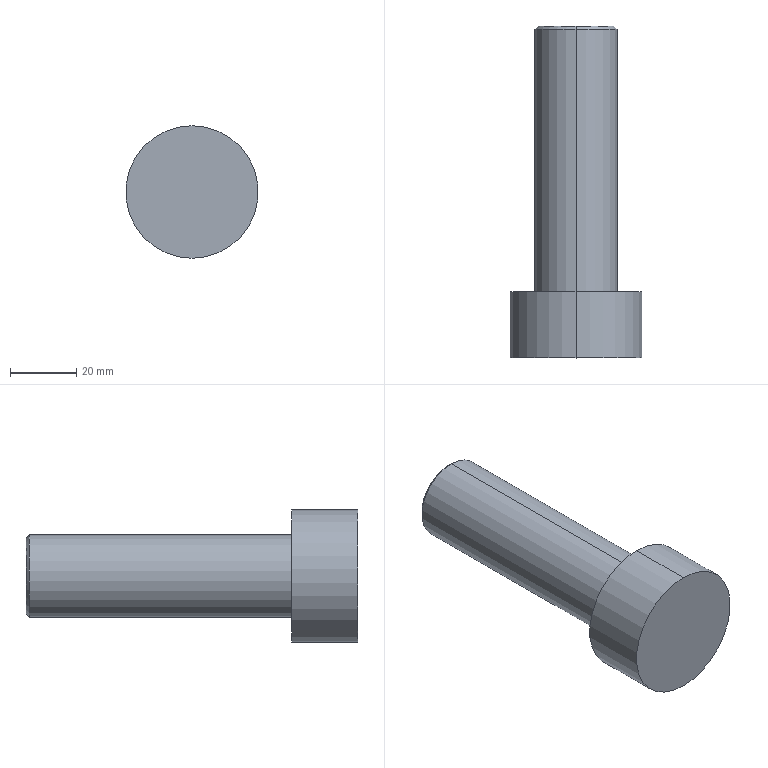Part | SolidWorks | features BaseBody 1, HoleWzd 1 | 1 solid | 13 faces | box 40 x 100.2 x 40 mm | volume 63721 mm3 | cylinder 6 | cone 4 | plane 3 | commonest cylinder face diameters 6.8 x2 25 x2 40 x2
STEP:
#1=CARTESIAN_POINT('',(0.,80.45,-3.4));
#2=VERTEX_POINT('',#1);
#3=CARTESIAN_POINT('',(0.,80.45,3.4));
#4=VERTEX_POINT('',#3);
#5=CARTESIAN_POINT('',(0.,80.45,0.));
#6=DIRECTION('',(0.,1.,0.));
#7=DIRECTION('',(0.,0.,1.));
#8=AXIS2_PLACEMENT_3D('',#5,#6,#7);
#9=CIRCLE('',#8,3.4);
#10=EDGE_CURVE('',#2,#4,#9,.T.);
#11=ORIENTED_EDGE('',*,*,#10,.F.);
#12=CARTESIAN_POINT('',(0.,100.2,-3.4));
#13=VERTEX_POINT('',#12);
#14=CARTESIAN_POINT('',(0.,100.2,-3.4));
#15=DIRECTION('',(0.,1.,0.));
#16=VECTOR('',#15,1000.);
#17=LINE('',#14,#16);
#18=EDGE_CURVE('',#2,#13,#17,.T.);
#19=ORIENTED_EDGE('',*,*,#18,.T.);
#20=CARTESIAN_POINT('',(0.,100.2,3.4));
#21=VERTEX_POINT('',#20);
#22=CARTESIAN_POINT('',(0.,100.2,0.));
#23=DIRECTION('',(0.,1.,0.));
#24=DIRECTION('',(0.,0.,1.));
#25=AXIS2_PLACEMENT_3D('',#22,#23,#24);
#26=CIRCLE('',#25,3.4);
#27=EDGE_CURVE('',#13,#21,#26,.T.);
#28=ORIENTED_EDGE('',*,*,#27,.T.);
#29=CARTESIAN_POINT('',(0.,100.2,3.4));
#30=DIRECTION('',(0.,1.,0.));
#31=VECTOR('',#30,1000.);
#32=LINE('',#29,#31);
#33=EDGE_CURVE('',#4,#21,#32,.T.);
#34=ORIENTED_EDGE('',*,*,#33,.F.);
#35=EDGE_LOOP('',(#11,#19,#28,#34));
#36=FACE_OUTER_BOUND('',#35,.T.);
#37=CARTESIAN_POINT('',(0.,100.2,0.));
#38=DIRECTION('',(0.,1.,0.));
#39=DIRECTION('',(0.,0.,1.));
#40=AXIS2_PLACEMENT_3D('',#37,#38,#39);
#41=CYLINDRICAL_SURFACE('',#40,3.4);
#42=ADVANCED_FACE('',(#36),#41,.F.);
#43=CARTESIAN_POINT('',(0.,78.407,0.));
#44=VERTEX_POINT('',#43);
#45=CARTESIAN_POINT('',(0.,80.45,3.4));
#46=DIRECTION('',(0.,0.515,0.8572));
#47=VECTOR('',#46,1000.);
#48=LINE('',#45,#47);
#49=EDGE_CURVE('',#44,#4,#48,.T.);
#50=ORIENTED_EDGE('',*,*,#49,.F.);
#51=CARTESIAN_POINT('',(0.,80.45,-3.4));
#52=DIRECTION('',(0.,0.515,-0.8572));
#53=VECTOR('',#52,1000.);
#54=LINE('',#51,#53);
#55=EDGE_CURVE('',#44,#2,#54,.T.);
#56=ORIENTED_EDGE('',*,*,#55,.T.);
#57=ORIENTED_EDGE('',*,*,#10,.T.);
#58=EDGE_LOOP('',(#50,#56,#57));
#59=FACE_OUTER_BOUND('',#58,.T.);
#60=CARTESIAN_POINT('',(0.,80.45,0.));
#61=DIRECTION('',(0.,1.,0.));
#62=DIRECTION('',(0.,0.,1.));
#63=AXIS2_PLACEMENT_3D('',#60,#61,#62);
#64=CONICAL_SURFACE('',#63,3.4,1.03);
#65=ADVANCED_FACE('',(#59),#64,.F.);
#66=CARTESIAN_POINT('',(0.,20.,12.5));
#67=VERTEX_POINT('',#66);
#68=CARTESIAN_POINT('',(0.,20.,-12.5));
#69=VERTEX_POINT('',#68);
#70=CARTESIAN_POINT('',(0.,20.,0.));
#71=DIRECTION('',(0.,1.,0.));
#72=DIRECTION('',(0.,0.,1.));
#73=AXIS2_PLACEMENT_3D('',#70,#71,#72);
#74=CIRCLE('',#73,12.5);
#75=EDGE_CURVE('',#67,#69,#74,.T.);
#76=ORIENTED_EDGE('',*,*,#75,.T.);
#77=CARTESIAN_POINT('',(0.,99.2,-12.5));
#78=VERTEX_POINT('',#77);
#79=CARTESIAN_POINT('',(0.,0.,-12.5));
#80=DIRECTION('',(0.,1.,0.));
#81=VECTOR('',#80,1000.);
#82=LINE('',#79,#81);
#83=EDGE_CURVE('',#69,#78,#82,.T.);
#84=ORIENTED_EDGE('',*,*,#83,.T.);
#85=CARTESIAN_POINT('',(0.,99.2,12.5));
#86=VERTEX_POINT('',#85);
#87=CARTESIAN_POINT('',(0.,99.2,0.));
#88=DIRECTION('',(0.,-1.,0.));
#89=DIRECTION('',(0.,0.,1.));
#90=AXIS2_PLACEMENT_3D('',#87,#88,#89);
#91=CIRCLE('',#90,12.5);
#92=EDGE_CURVE('',#78,#86,#91,.T.);
#93=ORIENTED_EDGE('',*,*,#92,.T.);
#94=CARTESIAN_POINT('',(0.,0.,12.5));
#95=DIRECTION('',(0.,1.,0.));
#96=VECTOR('',#95,1000.);
#97=LINE('',#94,#96);
#98=EDGE_CURVE('',#67,#86,#97,.T.);
#99=ORIENTED_EDGE('',*,*,#98,.F.);
#100=EDGE_LOOP('',(#76,#84,#93,#99));
#101=FACE_OUTER_BOUND('',#100,.T.);
#102=CARTESIAN_POINT('',(0.,0.,0.));
#103=DIRECTION('',(0.,1.,0.));
#104=DIRECTION('',(0.,0.,1.));
#105=AXIS2_PLACEMENT_3D('',#102,#103,#104);
#106=CYLINDRICAL_SURFACE('',#105,12.5);
#107=ADVANCED_FACE('',(#101),#106,.T.);
#108=CARTESIAN_POINT('',(0.,100.2,-11.5));
#109=VERTEX_POINT('',#108);
#110=CARTESIAN_POINT('',(0.,100.2,11.5));
#111=VERTEX_POINT('',#110);
#112=CARTESIAN_POINT('',(0.,100.2,0.));
#113=DIRECTION('',(0.,-1.,0.));
#114=DIRECTION('',(0.,0.,-1.));
#115=AXIS2_PLACEMENT_3D('',#112,#113,#114);
#116=CIRCLE('',#115,11.5);
#117=EDGE_CURVE('',#109,#111,#116,.T.);
#118=ORIENTED_EDGE('',*,*,#117,.T.);
#119=CARTESIAN_POINT('',(0.,99.2,12.5));
#120=DIRECTION('',(0.,-0.7071,0.7071));
#121=VECTOR('',#120,1000.);
#122=LINE('',#119,#121);
#123=EDGE_CURVE('',#111,#86,#122,.T.);
#124=ORIENTED_EDGE('',*,*,#123,.T.);
#125=ORIENTED_EDGE('',*,*,#92,.F.);
#126=CARTESIAN_POINT('',(0.,99.2,-12.5));
#127=DIRECTION('',(0.,-0.7071,-0.7071));
#128=VECTOR('',#127,1000.);
#129=LINE('',#126,#128);
#130=EDGE_CURVE('',#109,#78,#129,.T.);
#131=ORIENTED_EDGE('',*,*,#130,.F.);
#132=EDGE_LOOP('',(#118,#124,#125,#131));
#133=FACE_OUTER_BOUND('',#132,.T.);
#134=CARTESIAN_POINT('',(0.,99.2,0.));
#135=DIRECTION('',(0.,-1.,0.));
#136=DIRECTION('',(0.,0.,-1.));
#137=AXIS2_PLACEMENT_3D('',#134,#135,#136);
#138=CONICAL_SURFACE('',#137,12.5,0.7854);
#139=ADVANCED_FACE('',(#133),#138,.T.);
#140=CARTESIAN_POINT('',(0.,0.,20.));
#141=VERTEX_POINT('',#140);
#142=CARTESIAN_POINT('',(0.,0.,-20.));
#143=VERTEX_POINT('',#142);
#144=CARTESIAN_POINT('',(0.,0.,0.));
#145=DIRECTION('',(0.,1.,0.));
#146=DIRECTION('',(0.,0.,1.));
#147=AXIS2_PLACEMENT_3D('',#144,#145,#146);
#148=CIRCLE('',#147,20.);
#149=EDGE_CURVE('',#141,#143,#148,.T.);
#150=ORIENTED_EDGE('',*,*,#149,.T.);
#151=CARTESIAN_POINT('',(0.,20.,-20.));
#152=VERTEX_POINT('',#151);
#153=CARTESIAN_POINT('',(0.,0.,-20.));
#154=DIRECTION('',(0.,1.,0.));
#155=VECTOR('',#154,1000.);
#156=LINE('',#153,#155);
#157=EDGE_CURVE('',#143,#152,#156,.T.);
#158=ORIENTED_EDGE('',*,*,#157,.T.);
#159=CARTESIAN_POINT('',(0.,20.,20.));
#160=VERTEX_POINT('',#159);
#161=CARTESIAN_POINT('',(0.,20.,0.));
#162=DIRECTION('',(0.,-1.,0.));
#163=DIRECTION('',(0.,0.,1.));
#164=AXIS2_PLACEMENT_3D('',#161,#162,#163);
#165=CIRCLE('',#164,20.);
#166=EDGE_CURVE('',#152,#160,#165,.T.);
#167=ORIENTED_EDGE('',*,*,#166,.T.);
#168=CARTESIAN_POINT('',(0.,0.,20.));
#169=DIRECTION('',(0.,1.,0.));
#170=VECTOR('',#169,1000.);
#171=LINE('',#168,#170);
#172=EDGE_CURVE('',#141,#160,#171,.T.);
#173=ORIENTED_EDGE('',*,*,#172,.F.);
#174=EDGE_LOOP('',(#150,#158,#167,#173));
#175=FACE_OUTER_BOUND('',#174,.T.);
#176=CARTESIAN_POINT('',(0.,0.,0.));
#177=DIRECTION('',(0.,1.,0.));
#178=DIRECTION('',(0.,0.,1.));
#179=AXIS2_PLACEMENT_3D('',#176,#177,#178);
#180=CYLINDRICAL_SURFACE('',#179,20.);
#181=ADVANCED_FACE('',(#175),#180,.T.);
#182=ORIENTED_EDGE('',*,*,#83,.F.);
#183=CARTESIAN_POINT('',(0.,20.,0.));
#184=DIRECTION('',(0.,1.,0.));
#185=DIRECTION('',(0.,0.,1.));
#186=AXIS2_PLACEMENT_3D('',#183,#184,#185);
#187=CIRCLE('',#186,12.5);
#188=EDGE_CURVE('',#69,#67,#187,.T.);
#189=ORIENTED_EDGE('',*,*,#188,.T.);
#190=ORIENTED_EDGE('',*,*,#98,.T.);
#191=CARTESIAN_POINT('',(0.,99.2,0.));
#192=DIRECTION('',(0.,-1.,0.));
#193=DIRECTION('',(0.,0.,1.));
#194=AXIS2_PLACEMENT_3D('',#191,#192,#193);
#195=CIRCLE('',#194,12.5);
#196=EDGE_CURVE('',#86,#78,#195,.T.);
#197=ORIENTED_EDGE('',*,*,#196,.T.);
#198=EDGE_LOOP('',(#182,#189,#190,#197));
#199=FACE_OUTER_BOUND('',#198,.T.);
#200=CARTESIAN_POINT('',(0.,0.,0.));
#201=DIRECTION('',(0.,1.,0.));
#202=DIRECTION('',(0.,0.,1.));
#203=AXIS2_PLACEMENT_3D('',#200,#201,#202);
#204=CYLINDRICAL_SURFACE('',#203,12.5);
#205=ADVANCED_FACE('',(#199),#204,.T.);
#206=ORIENTED_EDGE('',*,*,#123,.F.);
#207=CARTESIAN_POINT('',(0.,100.2,0.));
#208=DIRECTION('',(0.,-1.,0.));
#209=DIRECTION('',(0.,0.,-1.));
#210=AXIS2_PLACEMENT_3D('',#207,#208,#209);
#211=CIRCLE('',#210,11.5);
#212=EDGE_CURVE('',#111,#109,#211,.T.);
#213=ORIENTED_EDGE('',*,*,#212,.T.);
#214=ORIENTED_EDGE('',*,*,#130,.T.);
#215=ORIENTED_EDGE('',*,*,#196,.F.);
#216=EDGE_LOOP('',(#206,#213,#214,#215));
#217=FACE_OUTER_BOUND('',#216,.T.);
#218=CARTESIAN_POINT('',(0.,99.2,0.));
#219=DIRECTION('',(0.,-1.,0.));
#220=DIRECTION('',(0.,0.,-1.));
#221=AXIS2_PLACEMENT_3D('',#218,#219,#220);
#222=CONICAL_SURFACE('',#221,12.5,0.7854);
#223=ADVANCED_FACE('',(#217),#222,.T.);
#224=ORIENTED_EDGE('',*,*,#75,.F.);
#225=ORIENTED_EDGE('',*,*,#188,.F.);
#226=EDGE_LOOP('',(#224,#225));
#227=FACE_BOUND('',#226,.T.);
#228=CARTESIAN_POINT('',(0.,20.,0.));
#229=DIRECTION('',(0.,-1.,0.));
#230=DIRECTION('',(0.,0.,1.));
#231=AXIS2_PLACEMENT_3D('',#228,#229,#230);
#232=CIRCLE('',#231,20.);
#233=EDGE_CURVE('',#160,#152,#232,.T.);
#234=ORIENTED_EDGE('',*,*,#233,.F.);
#235=ORIENTED_EDGE('',*,*,#166,.F.);
#236=EDGE_LOOP('',(#234,#235));
#237=FACE_OUTER_BOUND('',#236,.T.);
#238=CARTESIAN_POINT('',(12.5,20.,0.));
#239=DIRECTION('',(0.,-1.,0.));
#240=DIRECTION('',(0.,0.,-1.));
#241=AXIS2_PLACEMENT_3D('',#238,#239,#240);
#242=PLANE('',#241);
#243=ADVANCED_FACE('',(#227,#237),#242,.F.);
#244=CARTESIAN_POINT('',(0.,100.2,0.));
#245=DIRECTION('',(0.,1.,0.));
#246=DIRECTION('',(0.,0.,1.));
#247=AXIS2_PLACEMENT_3D('',#244,#245,#246);
#248=CIRCLE('',#247,3.4);
#249=EDGE_CURVE('',#21,#13,#248,.T.);
#250=ORIENTED_EDGE('',*,*,#249,.F.);
#251=ORIENTED_EDGE('',*,*,#27,.F.);
#252=EDGE_LOOP('',(#250,#251));
#253=FACE_BOUND('',#252,.T.);
#254=ORIENTED_EDGE('',*,*,#117,.F.);
#255=ORIENTED_EDGE('',*,*,#212,.F.);
#256=EDGE_LOOP('',(#254,#255));
#257=FACE_OUTER_BOUND('',#256,.T.);
#258=CARTESIAN_POINT('',(0.,100.2,0.));
#259=DIRECTION('',(0.,-1.,0.));
#260=DIRECTION('',(0.,0.,-1.));
#261=AXIS2_PLACEMENT_3D('',#258,#259,#260);
#262=PLANE('',#261);
#263=ADVANCED_FACE('',(#253,#257),#262,.F.);
#264=ORIENTED_EDGE('',*,*,#157,.F.);
#265=CARTESIAN_POINT('',(0.,0.,0.));
#266=DIRECTION('',(0.,1.,0.));
#267=DIRECTION('',(0.,0.,1.));
#268=AXIS2_PLACEMENT_3D('',#265,#266,#267);
#269=CIRCLE('',#268,20.);
#270=EDGE_CURVE('',#143,#141,#269,.T.);
#271=ORIENTED_EDGE('',*,*,#270,.T.);
#272=ORIENTED_EDGE('',*,*,#172,.T.);
#273=ORIENTED_EDGE('',*,*,#233,.T.);
#274=EDGE_LOOP('',(#264,#271,#272,#273));
#275=FACE_OUTER_BOUND('',#274,.T.);
#276=CARTESIAN_POINT('',(0.,0.,0.));
#277=DIRECTION('',(0.,1.,0.));
#278=DIRECTION('',(0.,0.,1.));
#279=AXIS2_PLACEMENT_3D('',#276,#277,#278);
#280=CYLINDRICAL_SURFACE('',#279,20.);
#281=ADVANCED_FACE('',(#275),#280,.T.);
#282=ORIENTED_EDGE('',*,*,#149,.F.);
#283=ORIENTED_EDGE('',*,*,#270,.F.);
#284=EDGE_LOOP('',(#282,#283));
#285=FACE_OUTER_BOUND('',#284,.T.);
#286=CARTESIAN_POINT('',(20.,0.,0.));
#287=DIRECTION('',(0.,1.,0.));
#288=DIRECTION('',(0.,0.,1.));
#289=AXIS2_PLACEMENT_3D('',#286,#287,#288);
#290=PLANE('',#289);
#291=ADVANCED_FACE('',(#285),#290,.F.);
#292=ORIENTED_EDGE('',*,*,#55,.F.);
#293=ORIENTED_EDGE('',*,*,#49,.T.);
#294=CARTESIAN_POINT('',(0.,80.45,0.));
#295=DIRECTION('',(0.,1.,0.));
#296=DIRECTION('',(0.,0.,1.));
#297=AXIS2_PLACEMENT_3D('',#294,#295,#296);
#298=CIRCLE('',#297,3.4);
#299=EDGE_CURVE('',#4,#2,#298,.T.);
#300=ORIENTED_EDGE('',*,*,#299,.T.);
#301=EDGE_LOOP('',(#292,#293,#300));
#302=FACE_OUTER_BOUND('',#301,.T.);
#303=CARTESIAN_POINT('',(0.,80.45,0.));
#304=DIRECTION('',(0.,1.,0.));
#305=DIRECTION('',(0.,0.,1.));
#306=AXIS2_PLACEMENT_3D('',#303,#304,#305);
#307=CONICAL_SURFACE('',#306,3.4,1.03);
#308=ADVANCED_FACE('',(#302),#307,.F.);
#309=ORIENTED_EDGE('',*,*,#18,.F.);
#310=ORIENTED_EDGE('',*,*,#299,.F.);
#311=ORIENTED_EDGE('',*,*,#33,.T.);
#312=ORIENTED_EDGE('',*,*,#249,.T.);
#313=EDGE_LOOP('',(#309,#310,#311,#312));
#314=FACE_OUTER_BOUND('',#313,.T.);
#315=CARTESIAN_POINT('',(0.,100.2,0.));
#316=DIRECTION('',(0.,1.,0.));
#317=DIRECTION('',(0.,0.,1.));
#318=AXIS2_PLACEMENT_3D('',#315,#316,#317);
#319=CYLINDRICAL_SURFACE('',#318,3.4);
#320=ADVANCED_FACE('',(#314),#319,.F.);
#321=CLOSED_SHELL('',(#42,#65,#107,#139,#181,#205,#223,#243,#263,#281,#291,#308,#320));
#322=MANIFOLD_SOLID_BREP('',#321);
#323=CARTESIAN_POINT('',(0.,0.,0.));
#324=DIRECTION('',(0.,0.,1.));
#325=DIRECTION('',(1.,0.,0.));
#326=AXIS2_PLACEMENT_3D('',#323,#324,#325);
#327=(LENGTH_UNIT()NAMED_UNIT(*)SI_UNIT(.MILLI.,.METRE.));
#328=UNCERTAINTY_MEASURE_WITH_UNIT(LENGTH_MEASURE(0.00001),#327,'','');
#329=(NAMED_UNIT(*)PLANE_ANGLE_UNIT()SI_UNIT($,.RADIAN.));
#330=(NAMED_UNIT(*)SI_UNIT($,.STERADIAN.)SOLID_ANGLE_UNIT());
#331=(GEOMETRIC_REPRESENTATION_CONTEXT(3)GLOBAL_UNCERTAINTY_ASSIGNED_CONTEXT((#328))GLOBAL_UNIT_ASSIGNED_CONTEXT((#327,#329,#330))REPRESENTATION_CONTEXT('',''));
#332=ADVANCED_BREP_SHAPE_REPRESENTATION('',(#322,#326),#331);